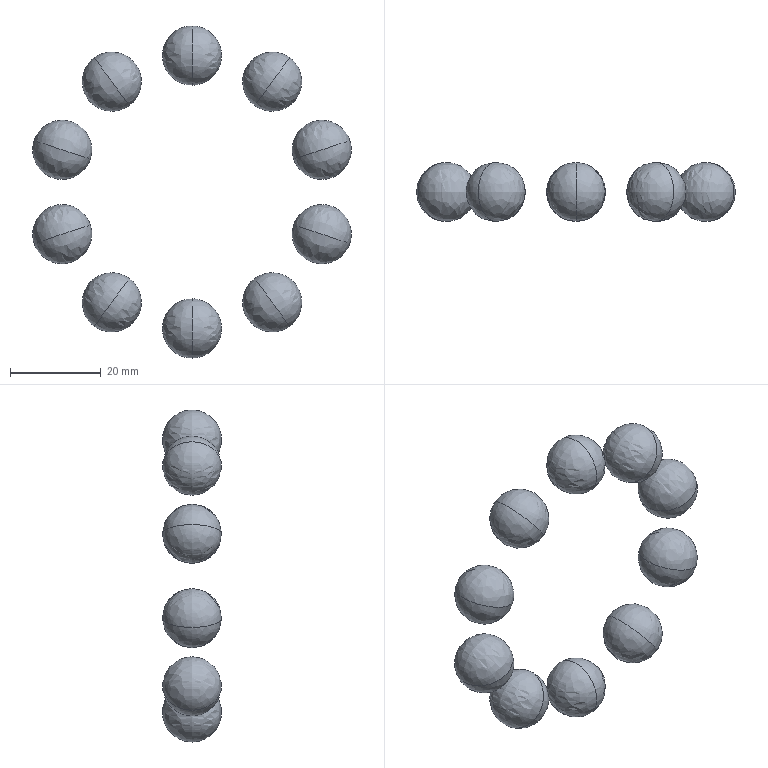Part | STEP file | Ball | 10 solids | 20 faces | box 70.063 x 13 x 73 mm | volume 11503 mm3 | spline 20
STEP:
#1=CARTESIAN_POINT('',(-13.813,0.,19.012));
#2=VERTEX_POINT('',#1);
#3=CARTESIAN_POINT('',(-21.454,0.,29.529));
#4=VERTEX_POINT('',#3);
#5=CARTESIAN_POINT('',(-17.634,0.,24.271));
#6=DIRECTION('',(0.809,0.,0.5878));
#7=DIRECTION('',(0.5878,0.,-0.809));
#8=AXIS2_PLACEMENT_3D('',#5,#6,#7);
#9=CIRCLE('',#8,6.5);
#10=EDGE_CURVE('',#2,#4,#9,.T.);
#11=ORIENTED_EDGE('',*,*,#10,.F.);
#12=CARTESIAN_POINT('',(-17.634,0.,24.271));
#13=DIRECTION('',(-0.809,0.,-0.5878));
#14=DIRECTION('',(0.5878,0.,-0.809));
#15=AXIS2_PLACEMENT_3D('',#12,#13,#14);
#16=CIRCLE('',#15,6.5);
#17=EDGE_CURVE('',#2,#4,#16,.T.);
#18=ORIENTED_EDGE('',*,*,#17,.T.);
#19=EDGE_LOOP('',(#11,#18));
#20=FACE_OUTER_BOUND('',#19,.T.);
#21=CARTESIAN_POINT('',(-13.813,0.,19.012));
#22=CARTESIAN_POINT('',(-13.813,0.,19.012));
#23=CARTESIAN_POINT('',(-13.813,0.,19.012));
#24=CARTESIAN_POINT('',(-13.813,0.,19.012));
#25=CARTESIAN_POINT('',(-13.813,-13.,19.012));
#26=CARTESIAN_POINT('',(-34.847,-13.,3.729));
#27=CARTESIAN_POINT('',(-34.847,13.,3.729));
#28=CARTESIAN_POINT('',(-13.813,13.,19.012));
#29=CARTESIAN_POINT('',(-21.454,-13.,29.529));
#30=CARTESIAN_POINT('',(-42.489,-13.,14.247));
#31=CARTESIAN_POINT('',(-42.489,13.,14.247));
#32=CARTESIAN_POINT('',(-21.454,13.,29.529));
#33=CARTESIAN_POINT('',(-21.454,0.,29.529));
#34=CARTESIAN_POINT('',(-21.454,0.,29.529));
#35=CARTESIAN_POINT('',(-21.454,0.,29.529));
#36=CARTESIAN_POINT('',(-21.454,0.,29.529));
#37=(BOUNDED_SURFACE()B_SPLINE_SURFACE(3,3,((#21,#22,#23,#24),(#25,#26,#27,#28),(#29,#30,#31,#32),(#33,#34,#35,#36)),.UNSPECIFIED.,.F.,.F.,.F.)B_SPLINE_SURFACE_WITH_KNOTS((4,4),(4,4),(0.,1.),(0.,1.),.UNSPECIFIED.)GEOMETRIC_REPRESENTATION_ITEM()RATIONAL_B_SPLINE_SURFACE(((1.,0.3333,0.3333,1.),(0.3333,0.1111,0.1111,0.3333),(0.3333,0.1111,0.1111,0.3333),(1.,0.3333,0.3333,1.)))REPRESENTATION_ITEM('')SURFACE());
#38=ADVANCED_FACE('',(#20),#37,.T.);
#39=ORIENTED_EDGE('',*,*,#17,.F.);
#40=ORIENTED_EDGE('',*,*,#10,.T.);
#41=EDGE_LOOP('',(#39,#40));
#42=FACE_OUTER_BOUND('',#41,.T.);
#43=CARTESIAN_POINT('',(-13.813,0.,19.012));
#44=CARTESIAN_POINT('',(-13.813,0.,19.012));
#45=CARTESIAN_POINT('',(-13.813,0.,19.012));
#46=CARTESIAN_POINT('',(-13.813,0.,19.012));
#47=CARTESIAN_POINT('',(-13.813,13.,19.012));
#48=CARTESIAN_POINT('',(7.221,13.,34.294));
#49=CARTESIAN_POINT('',(7.221,-13.,34.294));
#50=CARTESIAN_POINT('',(-13.813,-13.,19.012));
#51=CARTESIAN_POINT('',(-21.454,13.,29.529));
#52=CARTESIAN_POINT('',(-0.4197,13.,44.812));
#53=CARTESIAN_POINT('',(-0.4197,-13.,44.812));
#54=CARTESIAN_POINT('',(-21.454,-13.,29.529));
#55=CARTESIAN_POINT('',(-21.454,0.,29.529));
#56=CARTESIAN_POINT('',(-21.454,0.,29.529));
#57=CARTESIAN_POINT('',(-21.454,0.,29.529));
#58=CARTESIAN_POINT('',(-21.454,0.,29.529));
#59=(BOUNDED_SURFACE()B_SPLINE_SURFACE(3,3,((#43,#44,#45,#46),(#47,#48,#49,#50),(#51,#52,#53,#54),(#55,#56,#57,#58)),.UNSPECIFIED.,.F.,.F.,.F.)B_SPLINE_SURFACE_WITH_KNOTS((4,4),(4,4),(0.,1.),(0.,1.),.UNSPECIFIED.)GEOMETRIC_REPRESENTATION_ITEM()RATIONAL_B_SPLINE_SURFACE(((1.,0.3333,0.3333,1.),(0.3333,0.1111,0.1111,0.3333),(0.3333,0.1111,0.1111,0.3333),(1.,0.3333,0.3333,1.)))REPRESENTATION_ITEM('')SURFACE());
#60=ADVANCED_FACE('',(#42),#59,.T.);
#61=CLOSED_SHELL('',(#38,#60));
#62=MANIFOLD_SOLID_BREP('',#61);
#63=CARTESIAN_POINT('',(13.813,0.,19.012));
#64=VERTEX_POINT('',#63);
#65=CARTESIAN_POINT('',(21.454,0.,29.529));
#66=VERTEX_POINT('',#65);
#67=CARTESIAN_POINT('',(17.634,0.,24.271));
#68=DIRECTION('',(0.809,0.,-0.5878));
#69=DIRECTION('',(-0.5878,0.,-0.809));
#70=AXIS2_PLACEMENT_3D('',#67,#68,#69);
#71=CIRCLE('',#70,6.5);
#72=EDGE_CURVE('',#64,#66,#71,.T.);
#73=ORIENTED_EDGE('',*,*,#72,.F.);
#74=CARTESIAN_POINT('',(17.634,0.,24.271));
#75=DIRECTION('',(-0.809,0.,0.5878));
#76=DIRECTION('',(-0.5878,0.,-0.809));
#77=AXIS2_PLACEMENT_3D('',#74,#75,#76);
#78=CIRCLE('',#77,6.5);
#79=EDGE_CURVE('',#64,#66,#78,.T.);
#80=ORIENTED_EDGE('',*,*,#79,.T.);
#81=EDGE_LOOP('',(#73,#80));
#82=FACE_OUTER_BOUND('',#81,.T.);
#83=CARTESIAN_POINT('',(13.813,0.,19.012));
#84=CARTESIAN_POINT('',(13.813,0.,19.012));
#85=CARTESIAN_POINT('',(13.813,0.,19.012));
#86=CARTESIAN_POINT('',(13.813,0.,19.012));
#87=CARTESIAN_POINT('',(13.813,-13.,19.012));
#88=CARTESIAN_POINT('',(-7.221,-13.,34.294));
#89=CARTESIAN_POINT('',(-7.221,13.,34.294));
#90=CARTESIAN_POINT('',(13.813,13.,19.012));
#91=CARTESIAN_POINT('',(21.454,-13.,29.529));
#92=CARTESIAN_POINT('',(0.4197,-13.,44.812));
#93=CARTESIAN_POINT('',(0.4197,13.,44.812));
#94=CARTESIAN_POINT('',(21.454,13.,29.529));
#95=CARTESIAN_POINT('',(21.454,0.,29.529));
#96=CARTESIAN_POINT('',(21.454,0.,29.529));
#97=CARTESIAN_POINT('',(21.454,0.,29.529));
#98=CARTESIAN_POINT('',(21.454,0.,29.529));
#99=(BOUNDED_SURFACE()B_SPLINE_SURFACE(3,3,((#83,#84,#85,#86),(#87,#88,#89,#90),(#91,#92,#93,#94),(#95,#96,#97,#98)),.UNSPECIFIED.,.F.,.F.,.F.)B_SPLINE_SURFACE_WITH_KNOTS((4,4),(4,4),(0.,1.),(0.,1.),.UNSPECIFIED.)GEOMETRIC_REPRESENTATION_ITEM()RATIONAL_B_SPLINE_SURFACE(((1.,0.3333,0.3333,1.),(0.3333,0.1111,0.1111,0.3333),(0.3333,0.1111,0.1111,0.3333),(1.,0.3333,0.3333,1.)))REPRESENTATION_ITEM('')SURFACE());
#100=ADVANCED_FACE('',(#82),#99,.T.);
#101=ORIENTED_EDGE('',*,*,#79,.F.);
#102=ORIENTED_EDGE('',*,*,#72,.T.);
#103=EDGE_LOOP('',(#101,#102));
#104=FACE_OUTER_BOUND('',#103,.T.);
#105=CARTESIAN_POINT('',(13.813,0.,19.012));
#106=CARTESIAN_POINT('',(13.813,0.,19.012));
#107=CARTESIAN_POINT('',(13.813,0.,19.012));
#108=CARTESIAN_POINT('',(13.813,0.,19.012));
#109=CARTESIAN_POINT('',(13.813,13.,19.012));
#110=CARTESIAN_POINT('',(34.847,13.,3.729));
#111=CARTESIAN_POINT('',(34.847,-13.,3.729));
#112=CARTESIAN_POINT('',(13.813,-13.,19.012));
#113=CARTESIAN_POINT('',(21.454,13.,29.529));
#114=CARTESIAN_POINT('',(42.489,13.,14.247));
#115=CARTESIAN_POINT('',(42.489,-13.,14.247));
#116=CARTESIAN_POINT('',(21.454,-13.,29.529));
#117=CARTESIAN_POINT('',(21.454,0.,29.529));
#118=CARTESIAN_POINT('',(21.454,0.,29.529));
#119=CARTESIAN_POINT('',(21.454,0.,29.529));
#120=CARTESIAN_POINT('',(21.454,0.,29.529));
#121=(BOUNDED_SURFACE()B_SPLINE_SURFACE(3,3,((#105,#106,#107,#108),(#109,#110,#111,#112),(#113,#114,#115,#116),(#117,#118,#119,#120)),.UNSPECIFIED.,.F.,.F.,.F.)B_SPLINE_SURFACE_WITH_KNOTS((4,4),(4,4),(0.,1.),(0.,1.),.UNSPECIFIED.)GEOMETRIC_REPRESENTATION_ITEM()RATIONAL_B_SPLINE_SURFACE(((1.,0.3333,0.3333,1.),(0.3333,0.1111,0.1111,0.3333),(0.3333,0.1111,0.1111,0.3333),(1.,0.3333,0.3333,1.)))REPRESENTATION_ITEM('')SURFACE());
#122=ADVANCED_FACE('',(#104),#121,.T.);
#123=CLOSED_SHELL('',(#100,#122));
#124=MANIFOLD_SOLID_BREP('',#123);
#125=CARTESIAN_POINT('',(22.35,0.,7.262));
#126=VERTEX_POINT('',#125);
#127=CARTESIAN_POINT('',(34.714,0.,11.279));
#128=VERTEX_POINT('',#127);
#129=CARTESIAN_POINT('',(28.532,0.,9.271));
#130=DIRECTION('',(0.309,0.,-0.9511));
#131=DIRECTION('',(-0.9511,0.,-0.309));
#132=AXIS2_PLACEMENT_3D('',#129,#130,#131);
#133=CIRCLE('',#132,6.5);
#134=EDGE_CURVE('',#126,#128,#133,.T.);
#135=ORIENTED_EDGE('',*,*,#134,.F.);
#136=CARTESIAN_POINT('',(28.532,0.,9.271));
#137=DIRECTION('',(-0.309,0.,0.9511));
#138=DIRECTION('',(-0.9511,0.,-0.309));
#139=AXIS2_PLACEMENT_3D('',#136,#137,#138);
#140=CIRCLE('',#139,6.5);
#141=EDGE_CURVE('',#126,#128,#140,.T.);
#142=ORIENTED_EDGE('',*,*,#141,.T.);
#143=EDGE_LOOP('',(#135,#142));
#144=FACE_OUTER_BOUND('',#143,.T.);
#145=CARTESIAN_POINT('',(22.35,0.,7.262));
#146=CARTESIAN_POINT('',(22.35,0.,7.262));
#147=CARTESIAN_POINT('',(22.35,0.,7.262));
#148=CARTESIAN_POINT('',(22.35,0.,7.262));
#149=CARTESIAN_POINT('',(22.35,-13.,7.262));
#150=CARTESIAN_POINT('',(14.315,-13.,31.989));
#151=CARTESIAN_POINT('',(14.315,13.,31.989));
#152=CARTESIAN_POINT('',(22.35,13.,7.262));
#153=CARTESIAN_POINT('',(34.714,-13.,11.279));
#154=CARTESIAN_POINT('',(26.679,-13.,36.007));
#155=CARTESIAN_POINT('',(26.679,13.,36.007));
#156=CARTESIAN_POINT('',(34.714,13.,11.279));
#157=CARTESIAN_POINT('',(34.714,0.,11.279));
#158=CARTESIAN_POINT('',(34.714,0.,11.279));
#159=CARTESIAN_POINT('',(34.714,0.,11.279));
#160=CARTESIAN_POINT('',(34.714,0.,11.279));
#161=(BOUNDED_SURFACE()B_SPLINE_SURFACE(3,3,((#145,#146,#147,#148),(#149,#150,#151,#152),(#153,#154,#155,#156),(#157,#158,#159,#160)),.UNSPECIFIED.,.F.,.F.,.F.)B_SPLINE_SURFACE_WITH_KNOTS((4,4),(4,4),(0.,1.),(0.,1.),.UNSPECIFIED.)GEOMETRIC_REPRESENTATION_ITEM()RATIONAL_B_SPLINE_SURFACE(((1.,0.3333,0.3333,1.),(0.3333,0.1111,0.1111,0.3333),(0.3333,0.1111,0.1111,0.3333),(1.,0.3333,0.3333,1.)))REPRESENTATION_ITEM('')SURFACE());
#162=ADVANCED_FACE('',(#144),#161,.T.);
#163=ORIENTED_EDGE('',*,*,#141,.F.);
#164=ORIENTED_EDGE('',*,*,#134,.T.);
#165=EDGE_LOOP('',(#163,#164));
#166=FACE_OUTER_BOUND('',#165,.T.);
#167=CARTESIAN_POINT('',(22.35,0.,7.262));
#168=CARTESIAN_POINT('',(22.35,0.,7.262));
#169=CARTESIAN_POINT('',(22.35,0.,7.262));
#170=CARTESIAN_POINT('',(22.35,0.,7.262));
#171=CARTESIAN_POINT('',(22.35,13.,7.262));
#172=CARTESIAN_POINT('',(30.384,13.,-17.466));
#173=CARTESIAN_POINT('',(30.384,-13.,-17.466));
#174=CARTESIAN_POINT('',(22.35,-13.,7.262));
#175=CARTESIAN_POINT('',(34.714,13.,11.279));
#176=CARTESIAN_POINT('',(42.748,13.,-13.448));
#177=CARTESIAN_POINT('',(42.748,-13.,-13.448));
#178=CARTESIAN_POINT('',(34.714,-13.,11.279));
#179=CARTESIAN_POINT('',(34.714,0.,11.279));
#180=CARTESIAN_POINT('',(34.714,0.,11.279));
#181=CARTESIAN_POINT('',(34.714,0.,11.279));
#182=CARTESIAN_POINT('',(34.714,0.,11.279));
#183=(BOUNDED_SURFACE()B_SPLINE_SURFACE(3,3,((#167,#168,#169,#170),(#171,#172,#173,#174),(#175,#176,#177,#178),(#179,#180,#181,#182)),.UNSPECIFIED.,.F.,.F.,.F.)B_SPLINE_SURFACE_WITH_KNOTS((4,4),(4,4),(0.,1.),(0.,1.),.UNSPECIFIED.)GEOMETRIC_REPRESENTATION_ITEM()RATIONAL_B_SPLINE_SURFACE(((1.,0.3333,0.3333,1.),(0.3333,0.1111,0.1111,0.3333),(0.3333,0.1111,0.1111,0.3333),(1.,0.3333,0.3333,1.)))REPRESENTATION_ITEM('')SURFACE());
#184=ADVANCED_FACE('',(#166),#183,.T.);
#185=CLOSED_SHELL('',(#162,#184));
#186=MANIFOLD_SOLID_BREP('',#185);
#187=CARTESIAN_POINT('',(-13.813,0.,-19.012));
#188=VERTEX_POINT('',#187);
#189=CARTESIAN_POINT('',(-21.454,0.,-29.529));
#190=VERTEX_POINT('',#189);
#191=CARTESIAN_POINT('',(-17.634,0.,-24.271));
#192=DIRECTION('',(-0.809,0.,0.5878));
#193=DIRECTION('',(0.5878,0.,0.809));
#194=AXIS2_PLACEMENT_3D('',#191,#192,#193);
#195=CIRCLE('',#194,6.5);
#196=EDGE_CURVE('',#188,#190,#195,.T.);
#197=ORIENTED_EDGE('',*,*,#196,.F.);
#198=CARTESIAN_POINT('',(-17.634,0.,-24.271));
#199=DIRECTION('',(0.809,0.,-0.5878));
#200=DIRECTION('',(0.5878,0.,0.809));
#201=AXIS2_PLACEMENT_3D('',#198,#199,#200);
#202=CIRCLE('',#201,6.5);
#203=EDGE_CURVE('',#188,#190,#202,.T.);
#204=ORIENTED_EDGE('',*,*,#203,.T.);
#205=EDGE_LOOP('',(#197,#204));
#206=FACE_OUTER_BOUND('',#205,.T.);
#207=CARTESIAN_POINT('',(-13.813,0.,-19.012));
#208=CARTESIAN_POINT('',(-13.813,0.,-19.012));
#209=CARTESIAN_POINT('',(-13.813,0.,-19.012));
#210=CARTESIAN_POINT('',(-13.813,0.,-19.012));
#211=CARTESIAN_POINT('',(-13.813,-13.,-19.012));
#212=CARTESIAN_POINT('',(7.221,-13.,-34.294));
#213=CARTESIAN_POINT('',(7.221,13.,-34.294));
#214=CARTESIAN_POINT('',(-13.813,13.,-19.012));
#215=CARTESIAN_POINT('',(-21.454,-13.,-29.529));
#216=CARTESIAN_POINT('',(-0.4197,-13.,-44.812));
#217=CARTESIAN_POINT('',(-0.4197,13.,-44.812));
#218=CARTESIAN_POINT('',(-21.454,13.,-29.529));
#219=CARTESIAN_POINT('',(-21.454,0.,-29.529));
#220=CARTESIAN_POINT('',(-21.454,0.,-29.529));
#221=CARTESIAN_POINT('',(-21.454,0.,-29.529));
#222=CARTESIAN_POINT('',(-21.454,0.,-29.529));
#223=(BOUNDED_SURFACE()B_SPLINE_SURFACE(3,3,((#207,#208,#209,#210),(#211,#212,#213,#214),(#215,#216,#217,#218),(#219,#220,#221,#222)),.UNSPECIFIED.,.F.,.F.,.F.)B_SPLINE_SURFACE_WITH_KNOTS((4,4),(4,4),(0.,1.),(0.,1.),.UNSPECIFIED.)GEOMETRIC_REPRESENTATION_ITEM()RATIONAL_B_SPLINE_SURFACE(((1.,0.3333,0.3333,1.),(0.3333,0.1111,0.1111,0.3333),(0.3333,0.1111,0.1111,0.3333),(1.,0.3333,0.3333,1.)))REPRESENTATION_ITEM('')SURFACE());
#224=ADVANCED_FACE('',(#206),#223,.T.);
#225=ORIENTED_EDGE('',*,*,#203,.F.);
#226=ORIENTED_EDGE('',*,*,#196,.T.);
#227=EDGE_LOOP('',(#225,#226));
#228=FACE_OUTER_BOUND('',#227,.T.);
#229=CARTESIAN_POINT('',(-13.813,0.,-19.012));
#230=CARTESIAN_POINT('',(-13.813,0.,-19.012));
#231=CARTESIAN_POINT('',(-13.813,0.,-19.012));
#232=CARTESIAN_POINT('',(-13.813,0.,-19.012));
#233=CARTESIAN_POINT('',(-13.813,13.,-19.012));
#234=CARTESIAN_POINT('',(-34.847,13.,-3.729));
#235=CARTESIAN_POINT('',(-34.847,-13.,-3.729));
#236=CARTESIAN_POINT('',(-13.813,-13.,-19.012));
#237=CARTESIAN_POINT('',(-21.454,13.,-29.529));
#238=CARTESIAN_POINT('',(-42.489,13.,-14.247));
#239=CARTESIAN_POINT('',(-42.489,-13.,-14.247));
#240=CARTESIAN_POINT('',(-21.454,-13.,-29.529));
#241=CARTESIAN_POINT('',(-21.454,0.,-29.529));
#242=CARTESIAN_POINT('',(-21.454,0.,-29.529));
#243=CARTESIAN_POINT('',(-21.454,0.,-29.529));
#244=CARTESIAN_POINT('',(-21.454,0.,-29.529));
#245=(BOUNDED_SURFACE()B_SPLINE_SURFACE(3,3,((#229,#230,#231,#232),(#233,#234,#235,#236),(#237,#238,#239,#240),(#241,#242,#243,#244)),.UNSPECIFIED.,.F.,.F.,.F.)B_SPLINE_SURFACE_WITH_KNOTS((4,4),(4,4),(0.,1.),(0.,1.),.UNSPECIFIED.)GEOMETRIC_REPRESENTATION_ITEM()RATIONAL_B_SPLINE_SURFACE(((1.,0.3333,0.3333,1.),(0.3333,0.1111,0.1111,0.3333),(0.3333,0.1111,0.1111,0.3333),(1.,0.3333,0.3333,1.)))REPRESENTATION_ITEM('')SURFACE());
#246=ADVANCED_FACE('',(#228),#245,.T.);
#247=CLOSED_SHELL('',(#224,#246));
#248=MANIFOLD_SOLID_BREP('',#247);
#249=CARTESIAN_POINT('',(0.,0.,-23.5));
#250=VERTEX_POINT('',#249);
#251=CARTESIAN_POINT('',(0.,0.,-36.5));
#252=VERTEX_POINT('',#251);
#253=CARTESIAN_POINT('',(0.,0.,-30.));
#254=DIRECTION('',(-1.,0.,0.));
#255=DIRECTION('',(0.,0.,1.));
#256=AXIS2_PLACEMENT_3D('',#253,#254,#255);
#257=CIRCLE('',#256,6.5);
#258=EDGE_CURVE('',#250,#252,#257,.T.);
#259=ORIENTED_EDGE('',*,*,#258,.F.);
#260=CARTESIAN_POINT('',(0.,0.,-30.));
#261=DIRECTION('',(1.,0.,0.));
#262=DIRECTION('',(0.,0.,1.));
#263=AXIS2_PLACEMENT_3D('',#260,#261,#262);
#264=CIRCLE('',#263,6.5);
#265=EDGE_CURVE('',#250,#252,#264,.T.);
#266=ORIENTED_EDGE('',*,*,#265,.T.);
#267=EDGE_LOOP('',(#259,#266));
#268=FACE_OUTER_BOUND('',#267,.T.);
#269=CARTESIAN_POINT('',(0.,0.,-23.5));
#270=CARTESIAN_POINT('',(0.,0.,-23.5));
#271=CARTESIAN_POINT('',(0.,0.,-23.5));
#272=CARTESIAN_POINT('',(0.,0.,-23.5));
#273=CARTESIAN_POINT('',(0.,-13.,-23.5));
#274=CARTESIAN_POINT('',(26.,-13.,-23.5));
#275=CARTESIAN_POINT('',(26.,13.,-23.5));
#276=CARTESIAN_POINT('',(0.,13.,-23.5));
#277=CARTESIAN_POINT('',(0.,-13.,-36.5));
#278=CARTESIAN_POINT('',(26.,-13.,-36.5));
#279=CARTESIAN_POINT('',(26.,13.,-36.5));
#280=CARTESIAN_POINT('',(0.,13.,-36.5));
#281=CARTESIAN_POINT('',(0.,0.,-36.5));
#282=CARTESIAN_POINT('',(0.,0.,-36.5));
#283=CARTESIAN_POINT('',(0.,0.,-36.5));
#284=CARTESIAN_POINT('',(0.,0.,-36.5));
#285=(BOUNDED_SURFACE()B_SPLINE_SURFACE(3,3,((#269,#270,#271,#272),(#273,#274,#275,#276),(#277,#278,#279,#280),(#281,#282,#283,#284)),.UNSPECIFIED.,.F.,.F.,.F.)B_SPLINE_SURFACE_WITH_KNOTS((4,4),(4,4),(0.,1.),(0.,1.),.UNSPECIFIED.)GEOMETRIC_REPRESENTATION_ITEM()RATIONAL_B_SPLINE_SURFACE(((1.,0.3333,0.3333,1.),(0.3333,0.1111,0.1111,0.3333),(0.3333,0.1111,0.1111,0.3333),(1.,0.3333,0.3333,1.)))REPRESENTATION_ITEM('')SURFACE());
#286=ADVANCED_FACE('',(#268),#285,.T.);
#287=ORIENTED_EDGE('',*,*,#265,.F.);
#288=ORIENTED_EDGE('',*,*,#258,.T.);
#289=EDGE_LOOP('',(#287,#288));
#290=FACE_OUTER_BOUND('',#289,.T.);
#291=CARTESIAN_POINT('',(0.,0.,-23.5));
#292=CARTESIAN_POINT('',(0.,0.,-23.5));
#293=CARTESIAN_POINT('',(0.,0.,-23.5));
#294=CARTESIAN_POINT('',(0.,0.,-23.5));
#295=CARTESIAN_POINT('',(0.,13.,-23.5));
#296=CARTESIAN_POINT('',(-26.,13.,-23.5));
#297=CARTESIAN_POINT('',(-26.,-13.,-23.5));
#298=CARTESIAN_POINT('',(0.,-13.,-23.5));
#299=CARTESIAN_POINT('',(0.,13.,-36.5));
#300=CARTESIAN_POINT('',(-26.,13.,-36.5));
#301=CARTESIAN_POINT('',(-26.,-13.,-36.5));
#302=CARTESIAN_POINT('',(0.,-13.,-36.5));
#303=CARTESIAN_POINT('',(0.,0.,-36.5));
#304=CARTESIAN_POINT('',(0.,0.,-36.5));
#305=CARTESIAN_POINT('',(0.,0.,-36.5));
#306=CARTESIAN_POINT('',(0.,0.,-36.5));
#307=(BOUNDED_SURFACE()B_SPLINE_SURFACE(3,3,((#291,#292,#293,#294),(#295,#296,#297,#298),(#299,#300,#301,#302),(#303,#304,#305,#306)),.UNSPECIFIED.,.F.,.F.,.F.)B_SPLINE_SURFACE_WITH_KNOTS((4,4),(4,4),(0.,1.),(0.,1.),.UNSPECIFIED.)GEOMETRIC_REPRESENTATION_ITEM()RATIONAL_B_SPLINE_SURFACE(((1.,0.3333,0.3333,1.),(0.3333,0.1111,0.1111,0.3333),(0.3333,0.1111,0.1111,0.3333),(1.,0.3333,0.3333,1.)))REPRESENTATION_ITEM('')SURFACE());
#308=ADVANCED_FACE('',(#290),#307,.T.);
#309=CLOSED_SHELL('',(#286,#308));
#310=MANIFOLD_SOLID_BREP('',#309);
#311=CARTESIAN_POINT('',(13.813,0.,-19.012));
#312=VERTEX_POINT('',#311);
#313=CARTESIAN_POINT('',(21.454,0.,-29.529));
#314=VERTEX_POINT('',#313);
#315=CARTESIAN_POINT('',(17.634,0.,-24.271));
#316=DIRECTION('',(-0.809,0.,-0.5878));
#317=DIRECTION('',(-0.5878,0.,0.809));
#318=AXIS2_PLACEMENT_3D('',#315,#316,#317);
#319=CIRCLE('',#318,6.5);
#320=EDGE_CURVE('',#312,#314,#319,.T.);
#321=ORIENTED_EDGE('',*,*,#320,.F.);
#322=CARTESIAN_POINT('',(17.634,0.,-24.271));
#323=DIRECTION('',(0.809,0.,0.5878));
#324=DIRECTION('',(-0.5878,0.,0.809));
#325=AXIS2_PLACEMENT_3D('',#322,#323,#324);
#326=CIRCLE('',#325,6.5);
#327=EDGE_CURVE('',#312,#314,#326,.T.);
#328=ORIENTED_EDGE('',*,*,#327,.T.);
#329=EDGE_LOOP('',(#321,#328));
#330=FACE_OUTER_BOUND('',#329,.T.);
#331=CARTESIAN_POINT('',(13.813,0.,-19.012));
#332=CARTESIAN_POINT('',(13.813,0.,-19.012));
#333=CARTESIAN_POINT('',(13.813,0.,-19.012));
#334=CARTESIAN_POINT('',(13.813,0.,-19.012));
#335=CARTESIAN_POINT('',(13.813,-13.,-19.012));
#336=CARTESIAN_POINT('',(34.847,-13.,-3.729));
#337=CARTESIAN_POINT('',(34.847,13.,-3.729));
#338=CARTESIAN_POINT('',(13.813,13.,-19.012));
#339=CARTESIAN_POINT('',(21.454,-13.,-29.529));
#340=CARTESIAN_POINT('',(42.489,-13.,-14.247));
#341=CARTESIAN_POINT('',(42.489,13.,-14.247));
#342=CARTESIAN_POINT('',(21.454,13.,-29.529));
#343=CARTESIAN_POINT('',(21.454,0.,-29.529));
#344=CARTESIAN_POINT('',(21.454,0.,-29.529));
#345=CARTESIAN_POINT('',(21.454,0.,-29.529));
#346=CARTESIAN_POINT('',(21.454,0.,-29.529));
#347=(BOUNDED_SURFACE()B_SPLINE_SURFACE(3,3,((#331,#332,#333,#334),(#335,#336,#337,#338),(#339,#340,#341,#342),(#343,#344,#345,#346)),.UNSPECIFIED.,.F.,.F.,.F.)B_SPLINE_SURFACE_WITH_KNOTS((4,4),(4,4),(0.,1.),(0.,1.),.UNSPECIFIED.)GEOMETRIC_REPRESENTATION_ITEM()RATIONAL_B_SPLINE_SURFACE(((1.,0.3333,0.3333,1.),(0.3333,0.1111,0.1111,0.3333),(0.3333,0.1111,0.1111,0.3333),(1.,0.3333,0.3333,1.)))REPRESENTATION_ITEM('')SURFACE());
#348=ADVANCED_FACE('',(#330),#347,.T.);
#349=ORIENTED_EDGE('',*,*,#327,.F.);
#350=ORIENTED_EDGE('',*,*,#320,.T.);
#351=EDGE_LOOP('',(#349,#350));
#352=FACE_OUTER_BOUND('',#351,.T.);
#353=CARTESIAN_POINT('',(13.813,0.,-19.012));
#354=CARTESIAN_POINT('',(13.813,0.,-19.012));
#355=CARTESIAN_POINT('',(13.813,0.,-19.012));
#356=CARTESIAN_POINT('',(13.813,0.,-19.012));
#357=CARTESIAN_POINT('',(13.813,13.,-19.012));
#358=CARTESIAN_POINT('',(-7.221,13.,-34.294));
#359=CARTESIAN_POINT('',(-7.221,-13.,-34.294));
#360=CARTESIAN_POINT('',(13.813,-13.,-19.012));
#361=CARTESIAN_POINT('',(21.454,13.,-29.529));
#362=CARTESIAN_POINT('',(0.4197,13.,-44.812));
#363=CARTESIAN_POINT('',(0.4197,-13.,-44.812));
#364=CARTESIAN_POINT('',(21.454,-13.,-29.529));
#365=CARTESIAN_POINT('',(21.454,0.,-29.529));
#366=CARTESIAN_POINT('',(21.454,0.,-29.529));
#367=CARTESIAN_POINT('',(21.454,0.,-29.529));
#368=CARTESIAN_POINT('',(21.454,0.,-29.529));
#369=(BOUNDED_SURFACE()B_SPLINE_SURFACE(3,3,((#353,#354,#355,#356),(#357,#358,#359,#360),(#361,#362,#363,#364),(#365,#366,#367,#368)),.UNSPECIFIED.,.F.,.F.,.F.)B_SPLINE_SURFACE_WITH_KNOTS((4,4),(4,4),(0.,1.),(0.,1.),.UNSPECIFIED.)GEOMETRIC_REPRESENTATION_ITEM()RATIONAL_B_SPLINE_SURFACE(((1.,0.3333,0.3333,1.),(0.3333,0.1111,0.1111,0.3333),(0.3333,0.1111,0.1111,0.3333),(1.,0.3333,0.3333,1.)))REPRESENTATION_ITEM('')SURFACE());
#370=ADVANCED_FACE('',(#352),#369,.T.);
#371=CLOSED_SHELL('',(#348,#370));
#372=MANIFOLD_SOLID_BREP('',#371);
#373=CARTESIAN_POINT('',(22.35,0.,-7.262));
#374=VERTEX_POINT('',#373);
#375=CARTESIAN_POINT('',(34.714,0.,-11.279));
#376=VERTEX_POINT('',#375);
#377=CARTESIAN_POINT('',(28.532,0.,-9.271));
#378=DIRECTION('',(-0.309,0.,-0.9511));
#379=DIRECTION('',(-0.9511,0.,0.309));
#380=AXIS2_PLACEMENT_3D('',#377,#378,#379);
#381=CIRCLE('',#380,6.5);
#382=EDGE_CURVE('',#374,#376,#381,.T.);
#383=ORIENTED_EDGE('',*,*,#382,.F.);
#384=CARTESIAN_POINT('',(28.532,0.,-9.271));
#385=DIRECTION('',(0.309,0.,0.9511));
#386=DIRECTION('',(-0.9511,0.,0.309));
#387=AXIS2_PLACEMENT_3D('',#384,#385,#386);
#388=CIRCLE('',#387,6.5);
#389=EDGE_CURVE('',#374,#376,#388,.T.);
#390=ORIENTED_EDGE('',*,*,#389,.T.);
#391=EDGE_LOOP('',(#383,#390));
#392=FACE_OUTER_BOUND('',#391,.T.);
#393=CARTESIAN_POINT('',(22.35,0.,-7.262));
#394=CARTESIAN_POINT('',(22.35,0.,-7.262));
#395=CARTESIAN_POINT('',(22.35,0.,-7.262));
#396=CARTESIAN_POINT('',(22.35,0.,-7.262));
#397=CARTESIAN_POINT('',(22.35,-13.,-7.262));
#398=CARTESIAN_POINT('',(30.384,-13.,17.466));
#399=CARTESIAN_POINT('',(30.384,13.,17.466));
#400=CARTESIAN_POINT('',(22.35,13.,-7.262));
#401=CARTESIAN_POINT('',(34.714,-13.,-11.279));
#402=CARTESIAN_POINT('',(42.748,-13.,13.448));
#403=CARTESIAN_POINT('',(42.748,13.,13.448));
#404=CARTESIAN_POINT('',(34.714,13.,-11.279));
#405=CARTESIAN_POINT('',(34.714,0.,-11.279));
#406=CARTESIAN_POINT('',(34.714,0.,-11.279));
#407=CARTESIAN_POINT('',(34.714,0.,-11.279));
#408=CARTESIAN_POINT('',(34.714,0.,-11.279));
#409=(BOUNDED_SURFACE()B_SPLINE_SURFACE(3,3,((#393,#394,#395,#396),(#397,#398,#399,#400),(#401,#402,#403,#404),(#405,#406,#407,#408)),.UNSPECIFIED.,.F.,.F.,.F.)B_SPLINE_SURFACE_WITH_KNOTS((4,4),(4,4),(0.,1.),(0.,1.),.UNSPECIFIED.)GEOMETRIC_REPRESENTATION_ITEM()RATIONAL_B_SPLINE_SURFACE(((1.,0.3333,0.3333,1.),(0.3333,0.1111,0.1111,0.3333),(0.3333,0.1111,0.1111,0.3333),(1.,0.3333,0.3333,1.)))REPRESENTATION_ITEM('')SURFACE());
#410=ADVANCED_FACE('',(#392),#409,.T.);
#411=ORIENTED_EDGE('',*,*,#389,.F.);
#412=ORIENTED_EDGE('',*,*,#382,.T.);
#413=EDGE_LOOP('',(#411,#412));
#414=FACE_OUTER_BOUND('',#413,.T.);
#415=CARTESIAN_POINT('',(22.35,0.,-7.262));
#416=CARTESIAN_POINT('',(22.35,0.,-7.262));
#417=CARTESIAN_POINT('',(22.35,0.,-7.262));
#418=CARTESIAN_POINT('',(22.35,0.,-7.262));
#419=CARTESIAN_POINT('',(22.35,13.,-7.262));
#420=CARTESIAN_POINT('',(14.315,13.,-31.989));
#421=CARTESIAN_POINT('',(14.315,-13.,-31.989));
#422=CARTESIAN_POINT('',(22.35,-13.,-7.262));
#423=CARTESIAN_POINT('',(34.714,13.,-11.279));
#424=CARTESIAN_POINT('',(26.679,13.,-36.007));
#425=CARTESIAN_POINT('',(26.679,-13.,-36.007));
#426=CARTESIAN_POINT('',(34.714,-13.,-11.279));
#427=CARTESIAN_POINT('',(34.714,0.,-11.279));
#428=CARTESIAN_POINT('',(34.714,0.,-11.279));
#429=CARTESIAN_POINT('',(34.714,0.,-11.279));
#430=CARTESIAN_POINT('',(34.714,0.,-11.279));
#431=(BOUNDED_SURFACE()B_SPLINE_SURFACE(3,3,((#415,#416,#417,#418),(#419,#420,#421,#422),(#423,#424,#425,#426),(#427,#428,#429,#430)),.UNSPECIFIED.,.F.,.F.,.F.)B_SPLINE_SURFACE_WITH_KNOTS((4,4),(4,4),(0.,1.),(0.,1.),.UNSPECIFIED.)GEOMETRIC_REPRESENTATION_ITEM()RATIONAL_B_SPLINE_SURFACE(((1.,0.3333,0.3333,1.),(0.3333,0.1111,0.1111,0.3333),(0.3333,0.1111,0.1111,0.3333),(1.,0.3333,0.3333,1.)))REPRESENTATION_ITEM('')SURFACE());
#432=ADVANCED_FACE('',(#414),#431,.T.);
#433=CLOSED_SHELL('',(#410,#432));
#434=MANIFOLD_SOLID_BREP('',#433);
#435=CARTESIAN_POINT('',(-22.35,0.,-7.262));
#436=VERTEX_POINT('',#435);
#437=CARTESIAN_POINT('',(-34.714,0.,-11.279));
#438=VERTEX_POINT('',#437);
#439=CARTESIAN_POINT('',(-28.532,0.,-9.271));
#440=DIRECTION('',(-0.309,0.,0.9511));
#441=DIRECTION('',(0.9511,0.,0.309));
#442=AXIS2_PLACEMENT_3D('',#439,#440,#441);
#443=CIRCLE('',#442,6.5);
#444=EDGE_CURVE('',#436,#438,#443,.T.);
#445=ORIENTED_EDGE('',*,*,#444,.F.);
#446=CARTESIAN_POINT('',(-28.532,0.,-9.271));
#447=DIRECTION('',(0.309,0.,-0.9511));
#448=DIRECTION('',(0.9511,0.,0.309));
#449=AXIS2_PLACEMENT_3D('',#446,#447,#448);
#450=CIRCLE('',#449,6.5);
#451=EDGE_CURVE('',#436,#438,#450,.T.);
#452=ORIENTED_EDGE('',*,*,#451,.T.);
#453=EDGE_LOOP('',(#445,#452));
#454=FACE_OUTER_BOUND('',#453,.T.);
#455=CARTESIAN_POINT('',(-22.35,0.,-7.262));
#456=CARTESIAN_POINT('',(-22.35,0.,-7.262));
#457=CARTESIAN_POINT('',(-22.35,0.,-7.262));
#458=CARTESIAN_POINT('',(-22.35,0.,-7.262));
#459=CARTESIAN_POINT('',(-22.35,-13.,-7.262));
#460=CARTESIAN_POINT('',(-14.315,-13.,-31.989));
#461=CARTESIAN_POINT('',(-14.315,13.,-31.989));
#462=CARTESIAN_POINT('',(-22.35,13.,-7.262));
#463=CARTESIAN_POINT('',(-34.714,-13.,-11.279));
#464=CARTESIAN_POINT('',(-26.679,-13.,-36.007));
#465=CARTESIAN_POINT('',(-26.679,13.,-36.007));
#466=CARTESIAN_POINT('',(-34.714,13.,-11.279));
#467=CARTESIAN_POINT('',(-34.714,0.,-11.279));
#468=CARTESIAN_POINT('',(-34.714,0.,-11.279));
#469=CARTESIAN_POINT('',(-34.714,0.,-11.279));
#470=CARTESIAN_POINT('',(-34.714,0.,-11.279));
#471=(BOUNDED_SURFACE()B_SPLINE_SURFACE(3,3,((#455,#456,#457,#458),(#459,#460,#461,#462),(#463,#464,#465,#466),(#467,#468,#469,#470)),.UNSPECIFIED.,.F.,.F.,.F.)B_SPLINE_SURFACE_WITH_KNOTS((4,4),(4,4),(0.,1.),(0.,1.),.UNSPECIFIED.)GEOMETRIC_REPRESENTATION_ITEM()RATIONAL_B_SPLINE_SURFACE(((1.,0.3333,0.3333,1.),(0.3333,0.1111,0.1111,0.3333),(0.3333,0.1111,0.1111,0.3333),(1.,0.3333,0.3333,1.)))REPRESENTATION_ITEM('')SURFACE());
#472=ADVANCED_FACE('',(#454),#471,.T.);
#473=ORIENTED_EDGE('',*,*,#451,.F.);
#474=ORIENTED_EDGE('',*,*,#444,.T.);
#475=EDGE_LOOP('',(#473,#474));
#476=FACE_OUTER_BOUND('',#475,.T.);
#477=CARTESIAN_POINT('',(-22.35,0.,-7.262));
#478=CARTESIAN_POINT('',(-22.35,0.,-7.262));
#479=CARTESIAN_POINT('',(-22.35,0.,-7.262));
#480=CARTESIAN_POINT('',(-22.35,0.,-7.262));
#481=CARTESIAN_POINT('',(-22.35,13.,-7.262));
#482=CARTESIAN_POINT('',(-30.384,13.,17.466));
#483=CARTESIAN_POINT('',(-30.384,-13.,17.466));
#484=CARTESIAN_POINT('',(-22.35,-13.,-7.262));
#485=CARTESIAN_POINT('',(-34.714,13.,-11.279));
#486=CARTESIAN_POINT('',(-42.748,13.,13.448));
#487=CARTESIAN_POINT('',(-42.748,-13.,13.448));
#488=CARTESIAN_POINT('',(-34.714,-13.,-11.279));
#489=CARTESIAN_POINT('',(-34.714,0.,-11.279));
#490=CARTESIAN_POINT('',(-34.714,0.,-11.279));
#491=CARTESIAN_POINT('',(-34.714,0.,-11.279));
#492=CARTESIAN_POINT('',(-34.714,0.,-11.279));
#493=(BOUNDED_SURFACE()B_SPLINE_SURFACE(3,3,((#477,#478,#479,#480),(#481,#482,#483,#484),(#485,#486,#487,#488),(#489,#490,#491,#492)),.UNSPECIFIED.,.F.,.F.,.F.)B_SPLINE_SURFACE_WITH_KNOTS((4,4),(4,4),(0.,1.),(0.,1.),.UNSPECIFIED.)GEOMETRIC_REPRESENTATION_ITEM()RATIONAL_B_SPLINE_SURFACE(((1.,0.3333,0.3333,1.),(0.3333,0.1111,0.1111,0.3333),(0.3333,0.1111,0.1111,0.3333),(1.,0.3333,0.3333,1.)))REPRESENTATION_ITEM('')SURFACE());
#494=ADVANCED_FACE('',(#476),#493,.T.);
#495=CLOSED_SHELL('',(#472,#494));
#496=MANIFOLD_SOLID_BREP('',#495);
#497=CARTESIAN_POINT('',(0.,0.,23.5));
#498=VERTEX_POINT('',#497);
#499=CARTESIAN_POINT('',(0.,0.,36.5));
#500=VERTEX_POINT('',#499);
#501=CARTESIAN_POINT('',(0.,0.,30.));
#502=DIRECTION('',(1.,0.,0.));
#503=DIRECTION('',(0.,0.,-1.));
#504=AXIS2_PLACEMENT_3D('',#501,#502,#503);
#505=CIRCLE('',#504,6.5);
#506=EDGE_CURVE('',#498,#500,#505,.T.);
#507=ORIENTED_EDGE('',*,*,#506,.F.);
#508=CARTESIAN_POINT('',(0.,0.,30.));
#509=DIRECTION('',(-1.,0.,0.));
#510=DIRECTION('',(0.,0.,-1.));
#511=AXIS2_PLACEMENT_3D('',#508,#509,#510);
#512=CIRCLE('',#511,6.5);
#513=EDGE_CURVE('',#498,#500,#512,.T.);
#514=ORIENTED_EDGE('',*,*,#513,.T.);
#515=EDGE_LOOP('',(#507,#514));
#516=FACE_OUTER_BOUND('',#515,.T.);
#517=CARTESIAN_POINT('',(0.,0.,23.5));
#518=CARTESIAN_POINT('',(0.,0.,23.5));
#519=CARTESIAN_POINT('',(0.,0.,23.5));
#520=CARTESIAN_POINT('',(0.,0.,23.5));
#521=CARTESIAN_POINT('',(0.,-13.,23.5));
#522=CARTESIAN_POINT('',(-26.,-13.,23.5));
#523=CARTESIAN_POINT('',(-26.,13.,23.5));
#524=CARTESIAN_POINT('',(0.,13.,23.5));
#525=CARTESIAN_POINT('',(0.,-13.,36.5));
#526=CARTESIAN_POINT('',(-26.,-13.,36.5));
#527=CARTESIAN_POINT('',(-26.,13.,36.5));
#528=CARTESIAN_POINT('',(0.,13.,36.5));
#529=CARTESIAN_POINT('',(0.,0.,36.5));
#530=CARTESIAN_POINT('',(0.,0.,36.5));
#531=CARTESIAN_POINT('',(0.,0.,36.5));
#532=CARTESIAN_POINT('',(0.,0.,36.5));
#533=(BOUNDED_SURFACE()B_SPLINE_SURFACE(3,3,((#517,#518,#519,#520),(#521,#522,#523,#524),(#525,#526,#527,#528),(#529,#530,#531,#532)),.UNSPECIFIED.,.F.,.F.,.F.)B_SPLINE_SURFACE_WITH_KNOTS((4,4),(4,4),(0.,1.),(0.,1.),.UNSPECIFIED.)GEOMETRIC_REPRESENTATION_ITEM()RATIONAL_B_SPLINE_SURFACE(((1.,0.3333,0.3333,1.),(0.3333,0.1111,0.1111,0.3333),(0.3333,0.1111,0.1111,0.3333),(1.,0.3333,0.3333,1.)))REPRESENTATION_ITEM('')SURFACE());
#534=ADVANCED_FACE('',(#516),#533,.T.);
#535=ORIENTED_EDGE('',*,*,#513,.F.);
#536=ORIENTED_EDGE('',*,*,#506,.T.);
#537=EDGE_LOOP('',(#535,#536));
#538=FACE_OUTER_BOUND('',#537,.T.);
#539=CARTESIAN_POINT('',(0.,0.,23.5));
#540=CARTESIAN_POINT('',(0.,0.,23.5));
#541=CARTESIAN_POINT('',(0.,0.,23.5));
#542=CARTESIAN_POINT('',(0.,0.,23.5));
#543=CARTESIAN_POINT('',(0.,13.,23.5));
#544=CARTESIAN_POINT('',(26.,13.,23.5));
#545=CARTESIAN_POINT('',(26.,-13.,23.5));
#546=CARTESIAN_POINT('',(0.,-13.,23.5));
#547=CARTESIAN_POINT('',(0.,13.,36.5));
#548=CARTESIAN_POINT('',(26.,13.,36.5));
#549=CARTESIAN_POINT('',(26.,-13.,36.5));
#550=CARTESIAN_POINT('',(0.,-13.,36.5));
#551=CARTESIAN_POINT('',(0.,0.,36.5));
#552=CARTESIAN_POINT('',(0.,0.,36.5));
#553=CARTESIAN_POINT('',(0.,0.,36.5));
#554=CARTESIAN_POINT('',(0.,0.,36.5));
#555=(BOUNDED_SURFACE()B_SPLINE_SURFACE(3,3,((#539,#540,#541,#542),(#543,#544,#545,#546),(#547,#548,#549,#550),(#551,#552,#553,#554)),.UNSPECIFIED.,.F.,.F.,.F.)B_SPLINE_SURFACE_WITH_KNOTS((4,4),(4,4),(0.,1.),(0.,1.),.UNSPECIFIED.)GEOMETRIC_REPRESENTATION_ITEM()RATIONAL_B_SPLINE_SURFACE(((1.,0.3333,0.3333,1.),(0.3333,0.1111,0.1111,0.3333),(0.3333,0.1111,0.1111,0.3333),(1.,0.3333,0.3333,1.)))REPRESENTATION_ITEM('')SURFACE());
#556=ADVANCED_FACE('',(#538),#555,.T.);
#557=CLOSED_SHELL('',(#534,#556));
#558=MANIFOLD_SOLID_BREP('',#557);
#559=CARTESIAN_POINT('',(-22.35,0.,7.262));
#560=VERTEX_POINT('',#559);
#561=CARTESIAN_POINT('',(-34.714,0.,11.279));
#562=VERTEX_POINT('',#561);
#563=CARTESIAN_POINT('',(-28.532,0.,9.271));
#564=DIRECTION('',(0.309,0.,0.9511));
#565=DIRECTION('',(0.9511,0.,-0.309));
#566=AXIS2_PLACEMENT_3D('',#563,#564,#565);
#567=CIRCLE('',#566,6.5);
#568=EDGE_CURVE('',#560,#562,#567,.T.);
#569=ORIENTED_EDGE('',*,*,#568,.F.);
#570=CARTESIAN_POINT('',(-28.532,0.,9.271));
#571=DIRECTION('',(-0.309,0.,-0.9511));
#572=DIRECTION('',(0.9511,0.,-0.309));
#573=AXIS2_PLACEMENT_3D('',#570,#571,#572);
#574=CIRCLE('',#573,6.5);
#575=EDGE_CURVE('',#560,#562,#574,.T.);
#576=ORIENTED_EDGE('',*,*,#575,.T.);
#577=EDGE_LOOP('',(#569,#576));
#578=FACE_OUTER_BOUND('',#577,.T.);
#579=CARTESIAN_POINT('',(-22.35,0.,7.262));
#580=CARTESIAN_POINT('',(-22.35,0.,7.262));
#581=CARTESIAN_POINT('',(-22.35,0.,7.262));
#582=CARTESIAN_POINT('',(-22.35,0.,7.262));
#583=CARTESIAN_POINT('',(-22.35,-13.,7.262));
#584=CARTESIAN_POINT('',(-30.384,-13.,-17.466));
#585=CARTESIAN_POINT('',(-30.384,13.,-17.466));
#586=CARTESIAN_POINT('',(-22.35,13.,7.262));
#587=CARTESIAN_POINT('',(-34.714,-13.,11.279));
#588=CARTESIAN_POINT('',(-42.748,-13.,-13.448));
#589=CARTESIAN_POINT('',(-42.748,13.,-13.448));
#590=CARTESIAN_POINT('',(-34.714,13.,11.279));
#591=CARTESIAN_POINT('',(-34.714,0.,11.279));
#592=CARTESIAN_POINT('',(-34.714,0.,11.279));
#593=CARTESIAN_POINT('',(-34.714,0.,11.279));
#594=CARTESIAN_POINT('',(-34.714,0.,11.279));
#595=(BOUNDED_SURFACE()B_SPLINE_SURFACE(3,3,((#579,#580,#581,#582),(#583,#584,#585,#586),(#587,#588,#589,#590),(#591,#592,#593,#594)),.UNSPECIFIED.,.F.,.F.,.F.)B_SPLINE_SURFACE_WITH_KNOTS((4,4),(4,4),(0.,1.),(0.,1.),.UNSPECIFIED.)GEOMETRIC_REPRESENTATION_ITEM()RATIONAL_B_SPLINE_SURFACE(((1.,0.3333,0.3333,1.),(0.3333,0.1111,0.1111,0.3333),(0.3333,0.1111,0.1111,0.3333),(1.,0.3333,0.3333,1.)))REPRESENTATION_ITEM('')SURFACE());
#596=ADVANCED_FACE('',(#578),#595,.T.);
#597=ORIENTED_EDGE('',*,*,#575,.F.);
#598=ORIENTED_EDGE('',*,*,#568,.T.);
#599=EDGE_LOOP('',(#597,#598));
#600=FACE_OUTER_BOUND('',#599,.T.);
#601=CARTESIAN_POINT('',(-22.35,0.,7.262));
#602=CARTESIAN_POINT('',(-22.35,0.,7.262));
#603=CARTESIAN_POINT('',(-22.35,0.,7.262));
#604=CARTESIAN_POINT('',(-22.35,0.,7.262));
#605=CARTESIAN_POINT('',(-22.35,13.,7.262));
#606=CARTESIAN_POINT('',(-14.315,13.,31.989));
#607=CARTESIAN_POINT('',(-14.315,-13.,31.989));
#608=CARTESIAN_POINT('',(-22.35,-13.,7.262));
#609=CARTESIAN_POINT('',(-34.714,13.,11.279));
#610=CARTESIAN_POINT('',(-26.679,13.,36.007));
#611=CARTESIAN_POINT('',(-26.679,-13.,36.007));
#612=CARTESIAN_POINT('',(-34.714,-13.,11.279));
#613=CARTESIAN_POINT('',(-34.714,0.,11.279));
#614=CARTESIAN_POINT('',(-34.714,0.,11.279));
#615=CARTESIAN_POINT('',(-34.714,0.,11.279));
#616=CARTESIAN_POINT('',(-34.714,0.,11.279));
#617=(BOUNDED_SURFACE()B_SPLINE_SURFACE(3,3,((#601,#602,#603,#604),(#605,#606,#607,#608),(#609,#610,#611,#612),(#613,#614,#615,#616)),.UNSPECIFIED.,.F.,.F.,.F.)B_SPLINE_SURFACE_WITH_KNOTS((4,4),(4,4),(0.,1.),(0.,1.),.UNSPECIFIED.)GEOMETRIC_REPRESENTATION_ITEM()RATIONAL_B_SPLINE_SURFACE(((1.,0.3333,0.3333,1.),(0.3333,0.1111,0.1111,0.3333),(0.3333,0.1111,0.1111,0.3333),(1.,0.3333,0.3333,1.)))REPRESENTATION_ITEM('')SURFACE());
#618=ADVANCED_FACE('',(#600),#617,.T.);
#619=CLOSED_SHELL('',(#596,#618));
#620=MANIFOLD_SOLID_BREP('',#619);
#621=CARTESIAN_POINT('',(0.,0.,0.));
#622=DIRECTION('',(0.,0.,1.));
#623=DIRECTION('',(1.,0.,0.));
#624=AXIS2_PLACEMENT_3D('',#621,#622,#623);
#625=(LENGTH_UNIT()NAMED_UNIT(*)SI_UNIT(.MILLI.,.METRE.));
#626=UNCERTAINTY_MEASURE_WITH_UNIT(LENGTH_MEASURE(0.00001),#625,'','');
#627=(NAMED_UNIT(*)PLANE_ANGLE_UNIT()SI_UNIT($,.RADIAN.));
#628=(NAMED_UNIT(*)SI_UNIT($,.STERADIAN.)SOLID_ANGLE_UNIT());
#629=(GEOMETRIC_REPRESENTATION_CONTEXT(3)GLOBAL_UNCERTAINTY_ASSIGNED_CONTEXT((#626))GLOBAL_UNIT_ASSIGNED_CONTEXT((#625,#627,#628))REPRESENTATION_CONTEXT('',''));
#630=ADVANCED_BREP_SHAPE_REPRESENTATION('',(#62,#124,#186,#248,#310,#372,#434,#496,#558,#620,#624),#629);